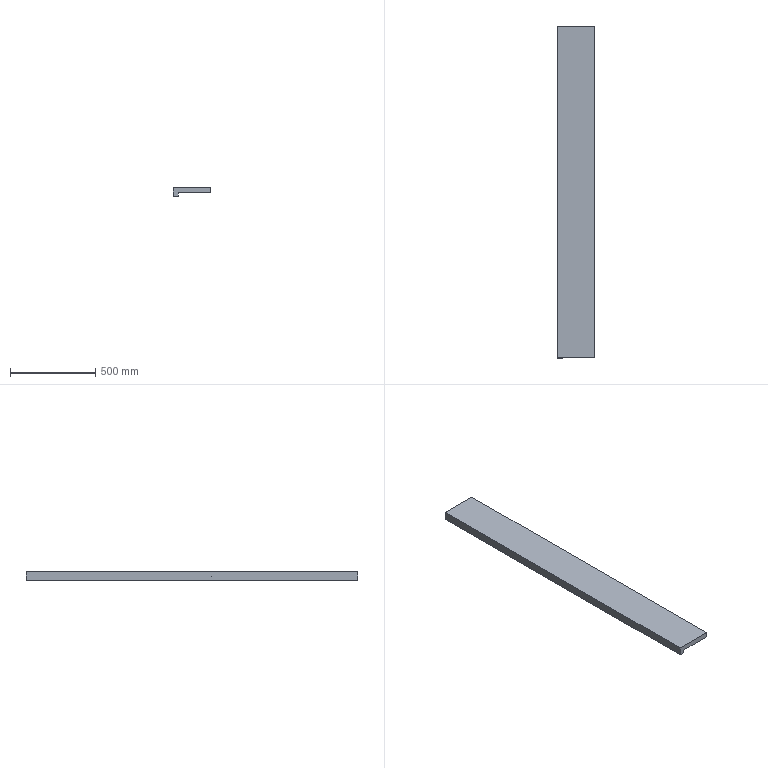Part | SolidWorks | features FlatPattern 1, ICE 1, SMBaseFlange 1, SheetMetal 1 | 1 solid | 8 faces | box 220 x 1950 x 50 mm | volume 14040000 mm3 | plane 8
STEP:
#1=CARTESIAN_POINT('',(110.,-975.,-30.));
#2=VERTEX_POINT('',#1);
#3=CARTESIAN_POINT('',(110.,-975.,0.));
#4=VERTEX_POINT('',#3);
#5=CARTESIAN_POINT('',(110.,-975.,-50.));
#6=DIRECTION('',(0.,0.,1.));
#7=VECTOR('',#6,1000.);
#8=LINE('',#5,#7);
#9=EDGE_CURVE('',#2,#4,#8,.T.);
#10=ORIENTED_EDGE('',*,*,#9,.F.);
#11=CARTESIAN_POINT('',(110.,975.,-30.));
#12=VERTEX_POINT('',#11);
#13=CARTESIAN_POINT('',(110.,975.,-30.));
#14=DIRECTION('',(0.,-1.,0.));
#15=VECTOR('',#14,1000.);
#16=LINE('',#13,#15);
#17=EDGE_CURVE('',#12,#2,#16,.T.);
#18=ORIENTED_EDGE('',*,*,#17,.F.);
#19=CARTESIAN_POINT('',(110.,975.,0.));
#20=VERTEX_POINT('',#19);
#21=CARTESIAN_POINT('',(110.,975.,-50.));
#22=DIRECTION('',(0.,0.,1.));
#23=VECTOR('',#22,1000.);
#24=LINE('',#21,#23);
#25=EDGE_CURVE('',#12,#20,#24,.T.);
#26=ORIENTED_EDGE('',*,*,#25,.T.);
#27=CARTESIAN_POINT('',(110.,975.,0.));
#28=DIRECTION('',(0.,1.,0.));
#29=VECTOR('',#28,1000.);
#30=LINE('',#27,#29);
#31=EDGE_CURVE('',#4,#20,#30,.T.);
#32=ORIENTED_EDGE('',*,*,#31,.F.);
#33=EDGE_LOOP('',(#10,#18,#26,#32));
#34=FACE_OUTER_BOUND('',#33,.T.);
#35=CARTESIAN_POINT('',(110.,975.,-50.));
#36=DIRECTION('',(1.,0.,0.));
#37=DIRECTION('',(0.,1.,0.));
#38=AXIS2_PLACEMENT_3D('',#35,#36,#37);
#39=PLANE('',#38);
#40=ADVANCED_FACE('',(#34),#39,.T.);
#41=CARTESIAN_POINT('',(-80.,-975.,-30.));
#42=VERTEX_POINT('',#41);
#43=CARTESIAN_POINT('',(-80.,-975.,-50.));
#44=VERTEX_POINT('',#43);
#45=CARTESIAN_POINT('',(-80.,-975.,-30.));
#46=DIRECTION('',(0.,0.,-1.));
#47=VECTOR('',#46,1000.);
#48=LINE('',#45,#47);
#49=EDGE_CURVE('',#42,#44,#48,.T.);
#50=ORIENTED_EDGE('',*,*,#49,.F.);
#51=CARTESIAN_POINT('',(110.,-975.,-30.));
#52=DIRECTION('',(-1.,0.,0.));
#53=VECTOR('',#52,1000.);
#54=LINE('',#51,#53);
#55=EDGE_CURVE('',#2,#42,#54,.T.);
#56=ORIENTED_EDGE('',*,*,#55,.F.);
#57=ORIENTED_EDGE('',*,*,#9,.T.);
#58=CARTESIAN_POINT('',(-110.,-975.,0.));
#59=VERTEX_POINT('',#58);
#60=CARTESIAN_POINT('',(-110.,-975.,0.));
#61=DIRECTION('',(1.,0.,0.));
#62=VECTOR('',#61,1000.);
#63=LINE('',#60,#62);
#64=EDGE_CURVE('',#59,#4,#63,.T.);
#65=ORIENTED_EDGE('',*,*,#64,.F.);
#66=CARTESIAN_POINT('',(-110.,-975.,-50.));
#67=VERTEX_POINT('',#66);
#68=CARTESIAN_POINT('',(-110.,-975.,-50.));
#69=DIRECTION('',(0.,0.,1.));
#70=VECTOR('',#69,1000.);
#71=LINE('',#68,#70);
#72=EDGE_CURVE('',#67,#59,#71,.T.);
#73=ORIENTED_EDGE('',*,*,#72,.F.);
#74=CARTESIAN_POINT('',(-110.,-975.,-50.));
#75=DIRECTION('',(1.,0.,0.));
#76=VECTOR('',#75,1000.);
#77=LINE('',#74,#76);
#78=EDGE_CURVE('',#67,#44,#77,.T.);
#79=ORIENTED_EDGE('',*,*,#78,.T.);
#80=EDGE_LOOP('',(#50,#56,#57,#65,#73,#79));
#81=FACE_OUTER_BOUND('',#80,.T.);
#82=CARTESIAN_POINT('',(-110.,-975.,-50.));
#83=DIRECTION('',(0.,-1.,0.));
#84=DIRECTION('',(0.,0.,-1.));
#85=AXIS2_PLACEMENT_3D('',#82,#83,#84);
#86=PLANE('',#85);
#87=ADVANCED_FACE('',(#81),#86,.T.);
#88=CARTESIAN_POINT('',(-110.,975.,0.));
#89=VERTEX_POINT('',#88);
#90=CARTESIAN_POINT('',(-110.,975.,0.));
#91=DIRECTION('',(0.,-1.,0.));
#92=VECTOR('',#91,1000.);
#93=LINE('',#90,#92);
#94=EDGE_CURVE('',#89,#59,#93,.T.);
#95=ORIENTED_EDGE('',*,*,#94,.F.);
#96=CARTESIAN_POINT('',(-110.,975.,-50.));
#97=VERTEX_POINT('',#96);
#98=CARTESIAN_POINT('',(-110.,975.,-50.));
#99=DIRECTION('',(0.,0.,1.));
#100=VECTOR('',#99,1000.);
#101=LINE('',#98,#100);
#102=EDGE_CURVE('',#97,#89,#101,.T.);
#103=ORIENTED_EDGE('',*,*,#102,.F.);
#104=CARTESIAN_POINT('',(-110.,975.,-50.));
#105=DIRECTION('',(0.,-1.,0.));
#106=VECTOR('',#105,1000.);
#107=LINE('',#104,#106);
#108=EDGE_CURVE('',#97,#67,#107,.T.);
#109=ORIENTED_EDGE('',*,*,#108,.T.);
#110=ORIENTED_EDGE('',*,*,#72,.T.);
#111=EDGE_LOOP('',(#95,#103,#109,#110));
#112=FACE_OUTER_BOUND('',#111,.T.);
#113=CARTESIAN_POINT('',(-110.,975.,-50.));
#114=DIRECTION('',(-1.,0.,0.));
#115=DIRECTION('',(0.,-1.,0.));
#116=AXIS2_PLACEMENT_3D('',#113,#114,#115);
#117=PLANE('',#116);
#118=ADVANCED_FACE('',(#112),#117,.T.);
#119=CARTESIAN_POINT('',(-80.,975.,-30.));
#120=VERTEX_POINT('',#119);
#121=CARTESIAN_POINT('',(-80.,975.,-50.));
#122=VERTEX_POINT('',#121);
#123=CARTESIAN_POINT('',(-80.,975.,-30.));
#124=DIRECTION('',(0.,0.,-1.));
#125=VECTOR('',#124,1000.);
#126=LINE('',#123,#125);
#127=EDGE_CURVE('',#120,#122,#126,.T.);
#128=ORIENTED_EDGE('',*,*,#127,.T.);
#129=CARTESIAN_POINT('',(-110.,975.,-50.));
#130=DIRECTION('',(-1.,0.,0.));
#131=VECTOR('',#130,1000.);
#132=LINE('',#129,#131);
#133=EDGE_CURVE('',#122,#97,#132,.T.);
#134=ORIENTED_EDGE('',*,*,#133,.T.);
#135=ORIENTED_EDGE('',*,*,#102,.T.);
#136=CARTESIAN_POINT('',(-110.,975.,0.));
#137=DIRECTION('',(-1.,0.,0.));
#138=VECTOR('',#137,1000.);
#139=LINE('',#136,#138);
#140=EDGE_CURVE('',#20,#89,#139,.T.);
#141=ORIENTED_EDGE('',*,*,#140,.F.);
#142=ORIENTED_EDGE('',*,*,#25,.F.);
#143=CARTESIAN_POINT('',(110.,975.,-30.));
#144=DIRECTION('',(1.,0.,0.));
#145=VECTOR('',#144,1000.);
#146=LINE('',#143,#145);
#147=EDGE_CURVE('',#120,#12,#146,.T.);
#148=ORIENTED_EDGE('',*,*,#147,.F.);
#149=EDGE_LOOP('',(#128,#134,#135,#141,#142,#148));
#150=FACE_OUTER_BOUND('',#149,.T.);
#151=CARTESIAN_POINT('',(-110.,975.,-50.));
#152=DIRECTION('',(0.,1.,0.));
#153=DIRECTION('',(0.,0.,1.));
#154=AXIS2_PLACEMENT_3D('',#151,#152,#153);
#155=PLANE('',#154);
#156=ADVANCED_FACE('',(#150),#155,.T.);
#157=ORIENTED_EDGE('',*,*,#133,.F.);
#158=CARTESIAN_POINT('',(-80.,975.,-50.));
#159=DIRECTION('',(0.,1.,0.));
#160=VECTOR('',#159,1000.);
#161=LINE('',#158,#160);
#162=EDGE_CURVE('',#44,#122,#161,.T.);
#163=ORIENTED_EDGE('',*,*,#162,.F.);
#164=ORIENTED_EDGE('',*,*,#78,.F.);
#165=ORIENTED_EDGE('',*,*,#108,.F.);
#166=EDGE_LOOP('',(#157,#163,#164,#165));
#167=FACE_OUTER_BOUND('',#166,.T.);
#168=CARTESIAN_POINT('',(0.,0.,-50.));
#169=DIRECTION('',(0.,0.,1.));
#170=DIRECTION('',(1.,0.,0.));
#171=AXIS2_PLACEMENT_3D('',#168,#169,#170);
#172=PLANE('',#171);
#173=ADVANCED_FACE('',(#167),#172,.F.);
#174=ORIENTED_EDGE('',*,*,#31,.T.);
#175=ORIENTED_EDGE('',*,*,#140,.T.);
#176=ORIENTED_EDGE('',*,*,#94,.T.);
#177=ORIENTED_EDGE('',*,*,#64,.T.);
#178=EDGE_LOOP('',(#174,#175,#176,#177));
#179=FACE_OUTER_BOUND('',#178,.T.);
#180=CARTESIAN_POINT('',(0.,0.,0.));
#181=DIRECTION('',(0.,0.,1.));
#182=DIRECTION('',(1.,0.,0.));
#183=AXIS2_PLACEMENT_3D('',#180,#181,#182);
#184=PLANE('',#183);
#185=ADVANCED_FACE('',(#179),#184,.T.);
#186=ORIENTED_EDGE('',*,*,#162,.T.);
#187=ORIENTED_EDGE('',*,*,#127,.F.);
#188=CARTESIAN_POINT('',(-80.,975.,-30.));
#189=DIRECTION('',(0.,1.,0.));
#190=VECTOR('',#189,1000.);
#191=LINE('',#188,#190);
#192=EDGE_CURVE('',#42,#120,#191,.T.);
#193=ORIENTED_EDGE('',*,*,#192,.F.);
#194=ORIENTED_EDGE('',*,*,#49,.T.);
#195=EDGE_LOOP('',(#186,#187,#193,#194));
#196=FACE_OUTER_BOUND('',#195,.T.);
#197=CARTESIAN_POINT('',(-80.,975.,-30.));
#198=DIRECTION('',(-1.,0.,0.));
#199=DIRECTION('',(0.,-1.,0.));
#200=AXIS2_PLACEMENT_3D('',#197,#198,#199);
#201=PLANE('',#200);
#202=ADVANCED_FACE('',(#196),#201,.F.);
#203=ORIENTED_EDGE('',*,*,#17,.T.);
#204=ORIENTED_EDGE('',*,*,#55,.T.);
#205=ORIENTED_EDGE('',*,*,#192,.T.);
#206=ORIENTED_EDGE('',*,*,#147,.T.);
#207=EDGE_LOOP('',(#203,#204,#205,#206));
#208=FACE_OUTER_BOUND('',#207,.T.);
#209=CARTESIAN_POINT('',(0.,0.,-30.));
#210=DIRECTION('',(0.,0.,-1.));
#211=DIRECTION('',(-1.,0.,0.));
#212=AXIS2_PLACEMENT_3D('',#209,#210,#211);
#213=PLANE('',#212);
#214=ADVANCED_FACE('',(#208),#213,.T.);
#215=CLOSED_SHELL('',(#40,#87,#118,#156,#173,#185,#202,#214));
#216=MANIFOLD_SOLID_BREP('',#215);
#217=CARTESIAN_POINT('',(0.,0.,0.));
#218=DIRECTION('',(0.,0.,1.));
#219=DIRECTION('',(1.,0.,0.));
#220=AXIS2_PLACEMENT_3D('',#217,#218,#219);
#221=(LENGTH_UNIT()NAMED_UNIT(*)SI_UNIT(.MILLI.,.METRE.));
#222=UNCERTAINTY_MEASURE_WITH_UNIT(LENGTH_MEASURE(0.00001),#221,'','');
#223=(NAMED_UNIT(*)PLANE_ANGLE_UNIT()SI_UNIT($,.RADIAN.));
#224=(NAMED_UNIT(*)SI_UNIT($,.STERADIAN.)SOLID_ANGLE_UNIT());
#225=(GEOMETRIC_REPRESENTATION_CONTEXT(3)GLOBAL_UNCERTAINTY_ASSIGNED_CONTEXT((#222))GLOBAL_UNIT_ASSIGNED_CONTEXT((#221,#223,#224))REPRESENTATION_CONTEXT('',''));
#226=ADVANCED_BREP_SHAPE_REPRESENTATION('',(#216,#220),#225);